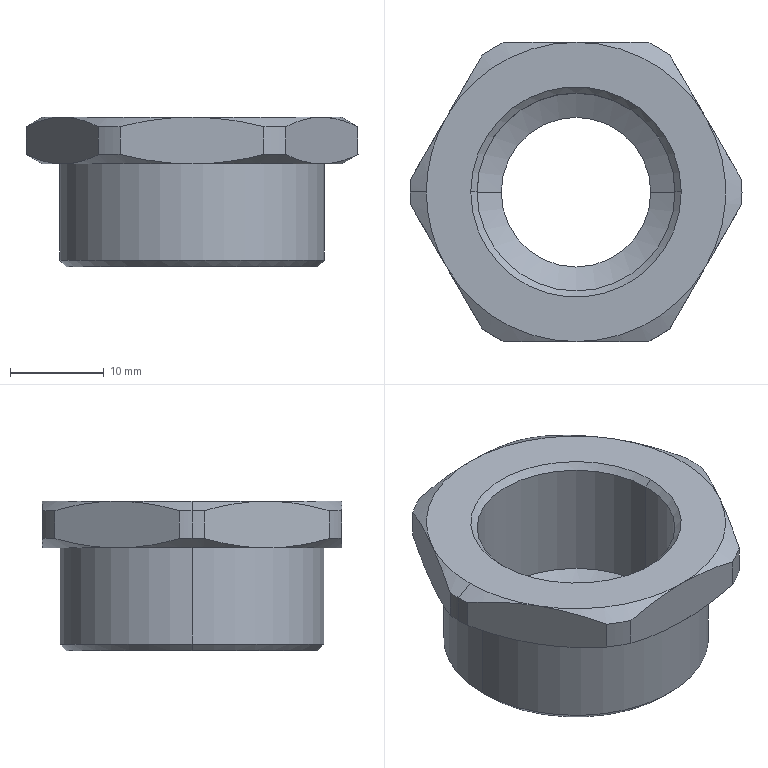Part | STEP file | 00193948_ADAPTERVERSCHR._MKA-PG-21-PG-16-KU.1 | 1 solid | 42 faces | box 35.5 x 32 x 16 mm | volume 5870 mm3 | cone 20 | cylinder 13 | plane 9 | commonest cylinder face diameters 35.5 x7 16 x2 21.16 x2 28.3 x2